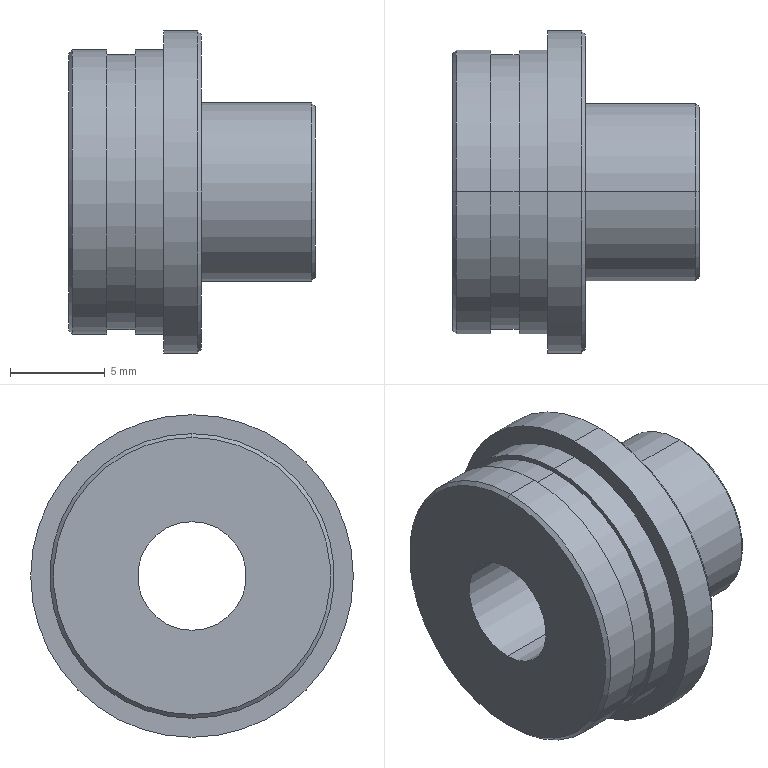Part | SolidWorks | features BaseBody 1 | 1 solid | 24 faces | box 13 x 17 x 17 mm | volume 1399 mm3 | cylinder 12 | cone 6 | plane 6 | commonest cylinder face diameters 15 x4 5.729 x2 9.4 x2 14.5 x2 17 x2
STEP:
#1=CARTESIAN_POINT('',(0.,0.,4.7));
#2=VERTEX_POINT('',#1);
#3=CARTESIAN_POINT('',(0.,0.,-4.7));
#4=VERTEX_POINT('',#3);
#5=CARTESIAN_POINT('',(0.,0.,0.));
#6=DIRECTION('',(-1.,0.,0.));
#7=DIRECTION('',(0.,0.,-1.));
#8=AXIS2_PLACEMENT_3D('',#5,#6,#7);
#9=CIRCLE('',#8,4.7);
#10=EDGE_CURVE('',#2,#4,#9,.T.);
#11=ORIENTED_EDGE('',*,*,#10,.F.);
#12=CARTESIAN_POINT('',(5.8,0.,4.7));
#13=VERTEX_POINT('',#12);
#14=CARTESIAN_POINT('',(0.,0.,4.7));
#15=DIRECTION('',(1.,0.,0.));
#16=VECTOR('',#15,1000.);
#17=LINE('',#14,#16);
#18=EDGE_CURVE('',#2,#13,#17,.T.);
#19=ORIENTED_EDGE('',*,*,#18,.T.);
#20=CARTESIAN_POINT('',(5.8,0.,-4.7));
#21=VERTEX_POINT('',#20);
#22=CARTESIAN_POINT('',(5.8,0.,0.));
#23=DIRECTION('',(-1.,0.,0.));
#24=DIRECTION('',(0.,0.,-1.));
#25=AXIS2_PLACEMENT_3D('',#22,#23,#24);
#26=CIRCLE('',#25,4.7);
#27=EDGE_CURVE('',#13,#21,#26,.T.);
#28=ORIENTED_EDGE('',*,*,#27,.T.);
#29=CARTESIAN_POINT('',(0.,0.,-4.7));
#30=DIRECTION('',(1.,0.,0.));
#31=VECTOR('',#30,1000.);
#32=LINE('',#29,#31);
#33=EDGE_CURVE('',#4,#21,#32,.T.);
#34=ORIENTED_EDGE('',*,*,#33,.F.);
#35=EDGE_LOOP('',(#11,#19,#28,#34));
#36=FACE_OUTER_BOUND('',#35,.T.);
#37=CARTESIAN_POINT('',(0.,0.,0.));
#38=DIRECTION('',(1.,0.,0.));
#39=DIRECTION('',(0.,0.,-1.));
#40=AXIS2_PLACEMENT_3D('',#37,#38,#39);
#41=CYLINDRICAL_SURFACE('',#40,4.7);
#42=ADVANCED_FACE('',(#36),#41,.T.);
#43=CARTESIAN_POINT('',(0.,0.,-8.3));
#44=VERTEX_POINT('',#43);
#45=CARTESIAN_POINT('',(0.,0.,8.3));
#46=VERTEX_POINT('',#45);
#47=CARTESIAN_POINT('',(0.,0.,0.));
#48=DIRECTION('',(1.,0.,0.));
#49=DIRECTION('',(0.,0.,1.));
#50=AXIS2_PLACEMENT_3D('',#47,#48,#49);
#51=CIRCLE('',#50,8.3);
#52=EDGE_CURVE('',#44,#46,#51,.T.);
#53=ORIENTED_EDGE('',*,*,#52,.F.);
#54=CARTESIAN_POINT('',(-0.2,0.,-8.5));
#55=VERTEX_POINT('',#54);
#56=CARTESIAN_POINT('',(-0.2,0.,-8.5));
#57=DIRECTION('',(-0.7071,0.,-0.7071));
#58=VECTOR('',#57,1000.);
#59=LINE('',#56,#58);
#60=EDGE_CURVE('',#44,#55,#59,.T.);
#61=ORIENTED_EDGE('',*,*,#60,.T.);
#62=CARTESIAN_POINT('',(-0.2,0.,8.5));
#63=VERTEX_POINT('',#62);
#64=CARTESIAN_POINT('',(-0.2,0.,0.));
#65=DIRECTION('',(1.,0.,0.));
#66=DIRECTION('',(0.,0.,1.));
#67=AXIS2_PLACEMENT_3D('',#64,#65,#66);
#68=CIRCLE('',#67,8.5);
#69=EDGE_CURVE('',#55,#63,#68,.T.);
#70=ORIENTED_EDGE('',*,*,#69,.T.);
#71=CARTESIAN_POINT('',(-0.2,0.,8.5));
#72=DIRECTION('',(-0.7071,0.,0.7071));
#73=VECTOR('',#72,1000.);
#74=LINE('',#71,#73);
#75=EDGE_CURVE('',#46,#63,#74,.T.);
#76=ORIENTED_EDGE('',*,*,#75,.F.);
#77=EDGE_LOOP('',(#53,#61,#70,#76));
#78=FACE_OUTER_BOUND('',#77,.T.);
#79=CARTESIAN_POINT('',(-0.2,0.,0.));
#80=DIRECTION('',(-1.,0.,0.));
#81=DIRECTION('',(0.,0.,1.));
#82=AXIS2_PLACEMENT_3D('',#79,#80,#81);
#83=CONICAL_SURFACE('',#82,8.5,0.7854);
#84=ADVANCED_FACE('',(#78),#83,.T.);
#85=CARTESIAN_POINT('',(6.,0.,4.5));
#86=VERTEX_POINT('',#85);
#87=CARTESIAN_POINT('',(6.,0.,-4.5));
#88=VERTEX_POINT('',#87);
#89=CARTESIAN_POINT('',(6.,0.,0.));
#90=DIRECTION('',(-1.,0.,0.));
#91=DIRECTION('',(0.,0.,1.));
#92=AXIS2_PLACEMENT_3D('',#89,#90,#91);
#93=CIRCLE('',#92,4.5);
#94=EDGE_CURVE('',#86,#88,#93,.T.);
#95=ORIENTED_EDGE('',*,*,#94,.T.);
#96=CARTESIAN_POINT('',(5.8,0.,-4.7));
#97=DIRECTION('',(-0.7071,0.,-0.7071));
#98=VECTOR('',#97,1000.);
#99=LINE('',#96,#98);
#100=EDGE_CURVE('',#88,#21,#99,.T.);
#101=ORIENTED_EDGE('',*,*,#100,.T.);
#102=ORIENTED_EDGE('',*,*,#27,.F.);
#103=CARTESIAN_POINT('',(5.8,0.,4.7));
#104=DIRECTION('',(-0.7071,0.,0.7071));
#105=VECTOR('',#104,1000.);
#106=LINE('',#103,#105);
#107=EDGE_CURVE('',#86,#13,#106,.T.);
#108=ORIENTED_EDGE('',*,*,#107,.F.);
#109=EDGE_LOOP('',(#95,#101,#102,#108));
#110=FACE_OUTER_BOUND('',#109,.T.);
#111=CARTESIAN_POINT('',(5.8,0.,0.));
#112=DIRECTION('',(-1.,0.,0.));
#113=DIRECTION('',(0.,0.,1.));
#114=AXIS2_PLACEMENT_3D('',#111,#112,#113);
#115=CONICAL_SURFACE('',#114,4.7,0.7854);
#116=ADVANCED_FACE('',(#110),#115,.T.);
#117=CARTESIAN_POINT('',(-2.,0.,-8.5));
#118=VERTEX_POINT('',#117);
#119=CARTESIAN_POINT('',(-2.,0.,8.5));
#120=VERTEX_POINT('',#119);
#121=CARTESIAN_POINT('',(-2.,0.,0.));
#122=DIRECTION('',(1.,0.,0.));
#123=DIRECTION('',(0.,0.,-1.));
#124=AXIS2_PLACEMENT_3D('',#121,#122,#123);
#125=CIRCLE('',#124,8.5);
#126=EDGE_CURVE('',#118,#120,#125,.T.);
#127=ORIENTED_EDGE('',*,*,#126,.T.);
#128=CARTESIAN_POINT('',(0.,0.,8.5));
#129=DIRECTION('',(1.,0.,0.));
#130=VECTOR('',#129,1000.);
#131=LINE('',#128,#130);
#132=EDGE_CURVE('',#120,#63,#131,.T.);
#133=ORIENTED_EDGE('',*,*,#132,.T.);
#134=ORIENTED_EDGE('',*,*,#69,.F.);
#135=CARTESIAN_POINT('',(0.,0.,-8.5));
#136=DIRECTION('',(1.,0.,0.));
#137=VECTOR('',#136,1000.);
#138=LINE('',#135,#137);
#139=EDGE_CURVE('',#118,#55,#138,.T.);
#140=ORIENTED_EDGE('',*,*,#139,.F.);
#141=EDGE_LOOP('',(#127,#133,#134,#140));
#142=FACE_OUTER_BOUND('',#141,.T.);
#143=CARTESIAN_POINT('',(0.,0.,0.));
#144=DIRECTION('',(1.,0.,0.));
#145=DIRECTION('',(0.,0.,-1.));
#146=AXIS2_PLACEMENT_3D('',#143,#144,#145);
#147=CYLINDRICAL_SURFACE('',#146,8.5);
#148=ADVANCED_FACE('',(#142),#147,.T.);
#149=CARTESIAN_POINT('',(-7.,0.,2.864));
#150=VERTEX_POINT('',#149);
#151=CARTESIAN_POINT('',(-7.,0.,-2.864));
#152=VERTEX_POINT('',#151);
#153=CARTESIAN_POINT('',(-7.,0.,0.));
#154=DIRECTION('',(1.,0.,0.));
#155=DIRECTION('',(0.,0.,-1.));
#156=AXIS2_PLACEMENT_3D('',#153,#154,#155);
#157=CIRCLE('',#156,2.864);
#158=EDGE_CURVE('',#150,#152,#157,.T.);
#159=ORIENTED_EDGE('',*,*,#158,.F.);
#160=CARTESIAN_POINT('',(6.,0.,2.864));
#161=VERTEX_POINT('',#160);
#162=CARTESIAN_POINT('',(0.,0.,2.864));
#163=DIRECTION('',(1.,0.,0.));
#164=VECTOR('',#163,1000.);
#165=LINE('',#162,#164);
#166=EDGE_CURVE('',#150,#161,#165,.T.);
#167=ORIENTED_EDGE('',*,*,#166,.T.);
#168=CARTESIAN_POINT('',(6.,0.,-2.864));
#169=VERTEX_POINT('',#168);
#170=CARTESIAN_POINT('',(6.,0.,0.));
#171=DIRECTION('',(-1.,0.,0.));
#172=DIRECTION('',(0.,0.,-1.));
#173=AXIS2_PLACEMENT_3D('',#170,#171,#172);
#174=CIRCLE('',#173,2.864);
#175=EDGE_CURVE('',#169,#161,#174,.T.);
#176=ORIENTED_EDGE('',*,*,#175,.F.);
#177=CARTESIAN_POINT('',(0.,0.,-2.864));
#178=DIRECTION('',(1.,0.,0.));
#179=VECTOR('',#178,1000.);
#180=LINE('',#177,#179);
#181=EDGE_CURVE('',#152,#169,#180,.T.);
#182=ORIENTED_EDGE('',*,*,#181,.F.);
#183=EDGE_LOOP('',(#159,#167,#176,#182));
#184=FACE_OUTER_BOUND('',#183,.T.);
#185=CARTESIAN_POINT('',(0.,0.,0.));
#186=DIRECTION('',(1.,0.,0.));
#187=DIRECTION('',(0.,0.,-1.));
#188=AXIS2_PLACEMENT_3D('',#185,#186,#187);
#189=CYLINDRICAL_SURFACE('',#188,2.864);
#190=ADVANCED_FACE('',(#184),#189,.F.);
#191=CARTESIAN_POINT('',(-3.5,0.,-7.5));
#192=VERTEX_POINT('',#191);
#193=CARTESIAN_POINT('',(-3.5,0.,7.5));
#194=VERTEX_POINT('',#193);
#195=CARTESIAN_POINT('',(-3.5,0.,0.));
#196=DIRECTION('',(1.,0.,0.));
#197=DIRECTION('',(0.,0.,-1.));
#198=AXIS2_PLACEMENT_3D('',#195,#196,#197);
#199=CIRCLE('',#198,7.5);
#200=EDGE_CURVE('',#192,#194,#199,.T.);
#201=ORIENTED_EDGE('',*,*,#200,.T.);
#202=CARTESIAN_POINT('',(-2.,0.,7.5));
#203=VERTEX_POINT('',#202);
#204=CARTESIAN_POINT('',(0.,0.,7.5));
#205=DIRECTION('',(1.,0.,0.));
#206=VECTOR('',#205,1000.);
#207=LINE('',#204,#206);
#208=EDGE_CURVE('',#194,#203,#207,.T.);
#209=ORIENTED_EDGE('',*,*,#208,.T.);
#210=CARTESIAN_POINT('',(-2.,0.,-7.5));
#211=VERTEX_POINT('',#210);
#212=CARTESIAN_POINT('',(-2.,0.,0.));
#213=DIRECTION('',(1.,0.,0.));
#214=DIRECTION('',(0.,0.,-1.));
#215=AXIS2_PLACEMENT_3D('',#212,#213,#214);
#216=CIRCLE('',#215,7.5);
#217=EDGE_CURVE('',#211,#203,#216,.T.);
#218=ORIENTED_EDGE('',*,*,#217,.F.);
#219=CARTESIAN_POINT('',(0.,0.,-7.5));
#220=DIRECTION('',(1.,0.,0.));
#221=VECTOR('',#220,1000.);
#222=LINE('',#219,#221);
#223=EDGE_CURVE('',#192,#211,#222,.T.);
#224=ORIENTED_EDGE('',*,*,#223,.F.);
#225=EDGE_LOOP('',(#201,#209,#218,#224));
#226=FACE_OUTER_BOUND('',#225,.T.);
#227=CARTESIAN_POINT('',(0.,0.,0.));
#228=DIRECTION('',(1.,0.,0.));
#229=DIRECTION('',(0.,0.,-1.));
#230=AXIS2_PLACEMENT_3D('',#227,#228,#229);
#231=CYLINDRICAL_SURFACE('',#230,7.5);
#232=ADVANCED_FACE('',(#226),#231,.T.);
#233=CARTESIAN_POINT('',(-7.,0.,7.3));
#234=VERTEX_POINT('',#233);
#235=CARTESIAN_POINT('',(-7.,0.,-7.3));
#236=VERTEX_POINT('',#235);
#237=CARTESIAN_POINT('',(-7.,0.,0.));
#238=DIRECTION('',(-1.,0.,0.));
#239=DIRECTION('',(0.,0.,-1.));
#240=AXIS2_PLACEMENT_3D('',#237,#238,#239);
#241=CIRCLE('',#240,7.3);
#242=EDGE_CURVE('',#234,#236,#241,.T.);
#243=ORIENTED_EDGE('',*,*,#242,.F.);
#244=CARTESIAN_POINT('',(-6.8,0.,7.5));
#245=VERTEX_POINT('',#244);
#246=CARTESIAN_POINT('',(-6.8,0.,7.5));
#247=DIRECTION('',(0.7071,0.,0.7071));
#248=VECTOR('',#247,1000.);
#249=LINE('',#246,#248);
#250=EDGE_CURVE('',#234,#245,#249,.T.);
#251=ORIENTED_EDGE('',*,*,#250,.T.);
#252=CARTESIAN_POINT('',(-6.8,0.,-7.5));
#253=VERTEX_POINT('',#252);
#254=CARTESIAN_POINT('',(-6.8,0.,0.));
#255=DIRECTION('',(-1.,0.,0.));
#256=DIRECTION('',(0.,0.,-1.));
#257=AXIS2_PLACEMENT_3D('',#254,#255,#256);
#258=CIRCLE('',#257,7.5);
#259=EDGE_CURVE('',#245,#253,#258,.T.);
#260=ORIENTED_EDGE('',*,*,#259,.T.);
#261=CARTESIAN_POINT('',(-6.8,0.,-7.5));
#262=DIRECTION('',(0.7071,0.,-0.7071));
#263=VECTOR('',#262,1000.);
#264=LINE('',#261,#263);
#265=EDGE_CURVE('',#236,#253,#264,.T.);
#266=ORIENTED_EDGE('',*,*,#265,.F.);
#267=EDGE_LOOP('',(#243,#251,#260,#266));
#268=FACE_OUTER_BOUND('',#267,.T.);
#269=CARTESIAN_POINT('',(-6.8,0.,0.));
#270=DIRECTION('',(1.,0.,0.));
#271=DIRECTION('',(0.,0.,-1.));
#272=AXIS2_PLACEMENT_3D('',#269,#270,#271);
#273=CONICAL_SURFACE('',#272,7.5,0.7854);
#274=ADVANCED_FACE('',(#268),#273,.T.);
#275=CARTESIAN_POINT('',(-5.,0.,-7.25));
#276=VERTEX_POINT('',#275);
#277=CARTESIAN_POINT('',(-5.,0.,7.25));
#278=VERTEX_POINT('',#277);
#279=CARTESIAN_POINT('',(-5.,0.,0.));
#280=DIRECTION('',(1.,0.,0.));
#281=DIRECTION('',(0.,0.,-1.));
#282=AXIS2_PLACEMENT_3D('',#279,#280,#281);
#283=CIRCLE('',#282,7.25);
#284=EDGE_CURVE('',#276,#278,#283,.T.);
#285=ORIENTED_EDGE('',*,*,#284,.T.);
#286=CARTESIAN_POINT('',(-3.5,0.,7.25));
#287=VERTEX_POINT('',#286);
#288=CARTESIAN_POINT('',(0.,0.,7.25));
#289=DIRECTION('',(1.,0.,0.));
#290=VECTOR('',#289,1000.);
#291=LINE('',#288,#290);
#292=EDGE_CURVE('',#278,#287,#291,.T.);
#293=ORIENTED_EDGE('',*,*,#292,.T.);
#294=CARTESIAN_POINT('',(-3.5,0.,-7.25));
#295=VERTEX_POINT('',#294);
#296=CARTESIAN_POINT('',(-3.5,0.,0.));
#297=DIRECTION('',(1.,0.,0.));
#298=DIRECTION('',(0.,0.,-1.));
#299=AXIS2_PLACEMENT_3D('',#296,#297,#298);
#300=CIRCLE('',#299,7.25);
#301=EDGE_CURVE('',#295,#287,#300,.T.);
#302=ORIENTED_EDGE('',*,*,#301,.F.);
#303=CARTESIAN_POINT('',(0.,0.,-7.25));
#304=DIRECTION('',(1.,0.,0.));
#305=VECTOR('',#304,1000.);
#306=LINE('',#303,#305);
#307=EDGE_CURVE('',#276,#295,#306,.T.);
#308=ORIENTED_EDGE('',*,*,#307,.F.);
#309=EDGE_LOOP('',(#285,#293,#302,#308));
#310=FACE_OUTER_BOUND('',#309,.T.);
#311=CARTESIAN_POINT('',(0.,0.,0.));
#312=DIRECTION('',(1.,0.,0.));
#313=DIRECTION('',(0.,0.,-1.));
#314=AXIS2_PLACEMENT_3D('',#311,#312,#313);
#315=CYLINDRICAL_SURFACE('',#314,7.25);
#316=ADVANCED_FACE('',(#310),#315,.T.);
#317=ORIENTED_EDGE('',*,*,#259,.F.);
#318=CARTESIAN_POINT('',(-5.,0.,7.5));
#319=VERTEX_POINT('',#318);
#320=CARTESIAN_POINT('',(0.,0.,7.5));
#321=DIRECTION('',(1.,0.,0.));
#322=VECTOR('',#321,1000.);
#323=LINE('',#320,#322);
#324=EDGE_CURVE('',#245,#319,#323,.T.);
#325=ORIENTED_EDGE('',*,*,#324,.T.);
#326=CARTESIAN_POINT('',(-5.,0.,-7.5));
#327=VERTEX_POINT('',#326);
#328=CARTESIAN_POINT('',(-5.,0.,0.));
#329=DIRECTION('',(-1.,0.,0.));
#330=DIRECTION('',(0.,0.,-1.));
#331=AXIS2_PLACEMENT_3D('',#328,#329,#330);
#332=CIRCLE('',#331,7.5);
#333=EDGE_CURVE('',#319,#327,#332,.T.);
#334=ORIENTED_EDGE('',*,*,#333,.T.);
#335=CARTESIAN_POINT('',(0.,0.,-7.5));
#336=DIRECTION('',(1.,0.,0.));
#337=VECTOR('',#336,1000.);
#338=LINE('',#335,#337);
#339=EDGE_CURVE('',#253,#327,#338,.T.);
#340=ORIENTED_EDGE('',*,*,#339,.F.);
#341=EDGE_LOOP('',(#317,#325,#334,#340));
#342=FACE_OUTER_BOUND('',#341,.T.);
#343=CARTESIAN_POINT('',(0.,0.,0.));
#344=DIRECTION('',(1.,0.,0.));
#345=DIRECTION('',(0.,0.,-1.));
#346=AXIS2_PLACEMENT_3D('',#343,#344,#345);
#347=CYLINDRICAL_SURFACE('',#346,7.5);
#348=ADVANCED_FACE('',(#342),#347,.T.);
#349=CARTESIAN_POINT('',(0.,0.,0.));
#350=DIRECTION('',(-1.,0.,0.));
#351=DIRECTION('',(0.,0.,-1.));
#352=AXIS2_PLACEMENT_3D('',#349,#350,#351);
#353=CIRCLE('',#352,4.7);
#354=EDGE_CURVE('',#4,#2,#353,.T.);
#355=ORIENTED_EDGE('',*,*,#354,.T.);
#356=ORIENTED_EDGE('',*,*,#10,.T.);
#357=EDGE_LOOP('',(#355,#356));
#358=FACE_BOUND('',#357,.T.);
#359=CARTESIAN_POINT('',(0.,0.,0.));
#360=DIRECTION('',(1.,0.,0.));
#361=DIRECTION('',(0.,0.,1.));
#362=AXIS2_PLACEMENT_3D('',#359,#360,#361);
#363=CIRCLE('',#362,8.3);
#364=EDGE_CURVE('',#46,#44,#363,.T.);
#365=ORIENTED_EDGE('',*,*,#364,.T.);
#366=ORIENTED_EDGE('',*,*,#52,.T.);
#367=EDGE_LOOP('',(#365,#366));
#368=FACE_OUTER_BOUND('',#367,.T.);
#369=CARTESIAN_POINT('',(0.,4.7,0.));
#370=DIRECTION('',(1.,0.,0.));
#371=DIRECTION('',(0.,0.,-1.));
#372=AXIS2_PLACEMENT_3D('',#369,#370,#371);
#373=PLANE('',#372);
#374=ADVANCED_FACE('',(#358,#368),#373,.T.);
#375=ORIENTED_EDGE('',*,*,#18,.F.);
#376=ORIENTED_EDGE('',*,*,#354,.F.);
#377=ORIENTED_EDGE('',*,*,#33,.T.);
#378=CARTESIAN_POINT('',(5.8,0.,0.));
#379=DIRECTION('',(-1.,0.,0.));
#380=DIRECTION('',(0.,0.,-1.));
#381=AXIS2_PLACEMENT_3D('',#378,#379,#380);
#382=CIRCLE('',#381,4.7);
#383=EDGE_CURVE('',#21,#13,#382,.T.);
#384=ORIENTED_EDGE('',*,*,#383,.T.);
#385=EDGE_LOOP('',(#375,#376,#377,#384));
#386=FACE_OUTER_BOUND('',#385,.T.);
#387=CARTESIAN_POINT('',(0.,0.,0.));
#388=DIRECTION('',(1.,0.,0.));
#389=DIRECTION('',(0.,0.,-1.));
#390=AXIS2_PLACEMENT_3D('',#387,#388,#389);
#391=CYLINDRICAL_SURFACE('',#390,4.7);
#392=ADVANCED_FACE('',(#386),#391,.T.);
#393=ORIENTED_EDGE('',*,*,#60,.F.);
#394=ORIENTED_EDGE('',*,*,#364,.F.);
#395=ORIENTED_EDGE('',*,*,#75,.T.);
#396=CARTESIAN_POINT('',(-0.2,0.,0.));
#397=DIRECTION('',(1.,0.,0.));
#398=DIRECTION('',(0.,0.,1.));
#399=AXIS2_PLACEMENT_3D('',#396,#397,#398);
#400=CIRCLE('',#399,8.5);
#401=EDGE_CURVE('',#63,#55,#400,.T.);
#402=ORIENTED_EDGE('',*,*,#401,.T.);
#403=EDGE_LOOP('',(#393,#394,#395,#402));
#404=FACE_OUTER_BOUND('',#403,.T.);
#405=CARTESIAN_POINT('',(-0.2,0.,0.));
#406=DIRECTION('',(-1.,0.,0.));
#407=DIRECTION('',(0.,0.,1.));
#408=AXIS2_PLACEMENT_3D('',#405,#406,#407);
#409=CONICAL_SURFACE('',#408,8.5,0.7854);
#410=ADVANCED_FACE('',(#404),#409,.T.);
#411=ORIENTED_EDGE('',*,*,#100,.F.);
#412=CARTESIAN_POINT('',(6.,0.,0.));
#413=DIRECTION('',(-1.,0.,0.));
#414=DIRECTION('',(0.,0.,1.));
#415=AXIS2_PLACEMENT_3D('',#412,#413,#414);
#416=CIRCLE('',#415,4.5);
#417=EDGE_CURVE('',#88,#86,#416,.T.);
#418=ORIENTED_EDGE('',*,*,#417,.T.);
#419=ORIENTED_EDGE('',*,*,#107,.T.);
#420=ORIENTED_EDGE('',*,*,#383,.F.);
#421=EDGE_LOOP('',(#411,#418,#419,#420));
#422=FACE_OUTER_BOUND('',#421,.T.);
#423=CARTESIAN_POINT('',(5.8,0.,0.));
#424=DIRECTION('',(-1.,0.,0.));
#425=DIRECTION('',(0.,0.,1.));
#426=AXIS2_PLACEMENT_3D('',#423,#424,#425);
#427=CONICAL_SURFACE('',#426,4.7,0.7854);
#428=ADVANCED_FACE('',(#422),#427,.T.);
#429=ORIENTED_EDGE('',*,*,#132,.F.);
#430=CARTESIAN_POINT('',(-2.,0.,0.));
#431=DIRECTION('',(1.,0.,0.));
#432=DIRECTION('',(0.,0.,-1.));
#433=AXIS2_PLACEMENT_3D('',#430,#431,#432);
#434=CIRCLE('',#433,8.5);
#435=EDGE_CURVE('',#120,#118,#434,.T.);
#436=ORIENTED_EDGE('',*,*,#435,.T.);
#437=ORIENTED_EDGE('',*,*,#139,.T.);
#438=ORIENTED_EDGE('',*,*,#401,.F.);
#439=EDGE_LOOP('',(#429,#436,#437,#438));
#440=FACE_OUTER_BOUND('',#439,.T.);
#441=CARTESIAN_POINT('',(0.,0.,0.));
#442=DIRECTION('',(1.,0.,0.));
#443=DIRECTION('',(0.,0.,-1.));
#444=AXIS2_PLACEMENT_3D('',#441,#442,#443);
#445=CYLINDRICAL_SURFACE('',#444,8.5);
#446=ADVANCED_FACE('',(#440),#445,.T.);
#447=ORIENTED_EDGE('',*,*,#175,.T.);
#448=CARTESIAN_POINT('',(6.,0.,0.));
#449=DIRECTION('',(-1.,0.,0.));
#450=DIRECTION('',(0.,0.,-1.));
#451=AXIS2_PLACEMENT_3D('',#448,#449,#450);
#452=CIRCLE('',#451,2.864);
#453=EDGE_CURVE('',#161,#169,#452,.T.);
#454=ORIENTED_EDGE('',*,*,#453,.T.);
#455=EDGE_LOOP('',(#447,#454));
#456=FACE_BOUND('',#455,.T.);
#457=ORIENTED_EDGE('',*,*,#94,.F.);
#458=ORIENTED_EDGE('',*,*,#417,.F.);
#459=EDGE_LOOP('',(#457,#458));
#460=FACE_OUTER_BOUND('',#459,.T.);
#461=CARTESIAN_POINT('',(6.,4.7,0.));
#462=DIRECTION('',(1.,0.,0.));
#463=DIRECTION('',(0.,0.,-1.));
#464=AXIS2_PLACEMENT_3D('',#461,#462,#463);
#465=PLANE('',#464);
#466=ADVANCED_FACE('',(#456,#460),#465,.T.);
#467=ORIENTED_EDGE('',*,*,#126,.F.);
#468=ORIENTED_EDGE('',*,*,#435,.F.);
#469=EDGE_LOOP('',(#467,#468));
#470=FACE_OUTER_BOUND('',#469,.T.);
#471=ORIENTED_EDGE('',*,*,#217,.T.);
#472=CARTESIAN_POINT('',(-2.,0.,0.));
#473=DIRECTION('',(1.,0.,0.));
#474=DIRECTION('',(0.,0.,-1.));
#475=AXIS2_PLACEMENT_3D('',#472,#473,#474);
#476=CIRCLE('',#475,7.5);
#477=EDGE_CURVE('',#203,#211,#476,.T.);
#478=ORIENTED_EDGE('',*,*,#477,.T.);
#479=EDGE_LOOP('',(#471,#478));
#480=FACE_BOUND('',#479,.T.);
#481=CARTESIAN_POINT('',(-2.,8.5,0.));
#482=DIRECTION('',(-1.,0.,0.));
#483=DIRECTION('',(0.,0.,1.));
#484=AXIS2_PLACEMENT_3D('',#481,#482,#483);
#485=PLANE('',#484);
#486=ADVANCED_FACE('',(#470,#480),#485,.T.);
#487=ORIENTED_EDGE('',*,*,#166,.F.);
#488=CARTESIAN_POINT('',(-7.,0.,0.));
#489=DIRECTION('',(1.,0.,0.));
#490=DIRECTION('',(0.,0.,-1.));
#491=AXIS2_PLACEMENT_3D('',#488,#489,#490);
#492=CIRCLE('',#491,2.864);
#493=EDGE_CURVE('',#152,#150,#492,.T.);
#494=ORIENTED_EDGE('',*,*,#493,.F.);
#495=ORIENTED_EDGE('',*,*,#181,.T.);
#496=ORIENTED_EDGE('',*,*,#453,.F.);
#497=EDGE_LOOP('',(#487,#494,#495,#496));
#498=FACE_OUTER_BOUND('',#497,.T.);
#499=CARTESIAN_POINT('',(0.,0.,0.));
#500=DIRECTION('',(1.,0.,0.));
#501=DIRECTION('',(0.,0.,-1.));
#502=AXIS2_PLACEMENT_3D('',#499,#500,#501);
#503=CYLINDRICAL_SURFACE('',#502,2.864);
#504=ADVANCED_FACE('',(#498),#503,.F.);
#505=ORIENTED_EDGE('',*,*,#208,.F.);
#506=CARTESIAN_POINT('',(-3.5,0.,0.));
#507=DIRECTION('',(1.,0.,0.));
#508=DIRECTION('',(0.,0.,-1.));
#509=AXIS2_PLACEMENT_3D('',#506,#507,#508);
#510=CIRCLE('',#509,7.5);
#511=EDGE_CURVE('',#194,#192,#510,.T.);
#512=ORIENTED_EDGE('',*,*,#511,.T.);
#513=ORIENTED_EDGE('',*,*,#223,.T.);
#514=ORIENTED_EDGE('',*,*,#477,.F.);
#515=EDGE_LOOP('',(#505,#512,#513,#514));
#516=FACE_OUTER_BOUND('',#515,.T.);
#517=CARTESIAN_POINT('',(0.,0.,0.));
#518=DIRECTION('',(1.,0.,0.));
#519=DIRECTION('',(0.,0.,-1.));
#520=AXIS2_PLACEMENT_3D('',#517,#518,#519);
#521=CYLINDRICAL_SURFACE('',#520,7.5);
#522=ADVANCED_FACE('',(#516),#521,.T.);
#523=ORIENTED_EDGE('',*,*,#493,.T.);
#524=ORIENTED_EDGE('',*,*,#158,.T.);
#525=EDGE_LOOP('',(#523,#524));
#526=FACE_BOUND('',#525,.T.);
#527=CARTESIAN_POINT('',(-7.,0.,0.));
#528=DIRECTION('',(-1.,0.,0.));
#529=DIRECTION('',(0.,0.,-1.));
#530=AXIS2_PLACEMENT_3D('',#527,#528,#529);
#531=CIRCLE('',#530,7.3);
#532=EDGE_CURVE('',#236,#234,#531,.T.);
#533=ORIENTED_EDGE('',*,*,#532,.T.);
#534=ORIENTED_EDGE('',*,*,#242,.T.);
#535=EDGE_LOOP('',(#533,#534));
#536=FACE_OUTER_BOUND('',#535,.T.);
#537=CARTESIAN_POINT('',(-7.,7.5,0.));
#538=DIRECTION('',(-1.,0.,0.));
#539=DIRECTION('',(0.,0.,1.));
#540=AXIS2_PLACEMENT_3D('',#537,#538,#539);
#541=PLANE('',#540);
#542=ADVANCED_FACE('',(#526,#536),#541,.T.);
#543=ORIENTED_EDGE('',*,*,#200,.F.);
#544=ORIENTED_EDGE('',*,*,#511,.F.);
#545=EDGE_LOOP('',(#543,#544));
#546=FACE_OUTER_BOUND('',#545,.T.);
#547=ORIENTED_EDGE('',*,*,#301,.T.);
#548=CARTESIAN_POINT('',(-3.5,0.,0.));
#549=DIRECTION('',(1.,0.,0.));
#550=DIRECTION('',(0.,0.,-1.));
#551=AXIS2_PLACEMENT_3D('',#548,#549,#550);
#552=CIRCLE('',#551,7.25);
#553=EDGE_CURVE('',#287,#295,#552,.T.);
#554=ORIENTED_EDGE('',*,*,#553,.T.);
#555=EDGE_LOOP('',(#547,#554));
#556=FACE_BOUND('',#555,.T.);
#557=CARTESIAN_POINT('',(-3.5,7.5,0.));
#558=DIRECTION('',(-1.,0.,0.));
#559=DIRECTION('',(0.,0.,1.));
#560=AXIS2_PLACEMENT_3D('',#557,#558,#559);
#561=PLANE('',#560);
#562=ADVANCED_FACE('',(#546,#556),#561,.T.);
#563=ORIENTED_EDGE('',*,*,#250,.F.);
#564=ORIENTED_EDGE('',*,*,#532,.F.);
#565=ORIENTED_EDGE('',*,*,#265,.T.);
#566=CARTESIAN_POINT('',(-6.8,0.,0.));
#567=DIRECTION('',(-1.,0.,0.));
#568=DIRECTION('',(0.,0.,-1.));
#569=AXIS2_PLACEMENT_3D('',#566,#567,#568);
#570=CIRCLE('',#569,7.5);
#571=EDGE_CURVE('',#253,#245,#570,.T.);
#572=ORIENTED_EDGE('',*,*,#571,.T.);
#573=EDGE_LOOP('',(#563,#564,#565,#572));
#574=FACE_OUTER_BOUND('',#573,.T.);
#575=CARTESIAN_POINT('',(-6.8,0.,0.));
#576=DIRECTION('',(1.,0.,0.));
#577=DIRECTION('',(0.,0.,-1.));
#578=AXIS2_PLACEMENT_3D('',#575,#576,#577);
#579=CONICAL_SURFACE('',#578,7.5,0.7854);
#580=ADVANCED_FACE('',(#574),#579,.T.);
#581=ORIENTED_EDGE('',*,*,#292,.F.);
#582=CARTESIAN_POINT('',(-5.,0.,0.));
#583=DIRECTION('',(1.,0.,0.));
#584=DIRECTION('',(0.,0.,-1.));
#585=AXIS2_PLACEMENT_3D('',#582,#583,#584);
#586=CIRCLE('',#585,7.25);
#587=EDGE_CURVE('',#278,#276,#586,.T.);
#588=ORIENTED_EDGE('',*,*,#587,.T.);
#589=ORIENTED_EDGE('',*,*,#307,.T.);
#590=ORIENTED_EDGE('',*,*,#553,.F.);
#591=EDGE_LOOP('',(#581,#588,#589,#590));
#592=FACE_OUTER_BOUND('',#591,.T.);
#593=CARTESIAN_POINT('',(0.,0.,0.));
#594=DIRECTION('',(1.,0.,0.));
#595=DIRECTION('',(0.,0.,-1.));
#596=AXIS2_PLACEMENT_3D('',#593,#594,#595);
#597=CYLINDRICAL_SURFACE('',#596,7.25);
#598=ADVANCED_FACE('',(#592),#597,.T.);
#599=ORIENTED_EDGE('',*,*,#324,.F.);
#600=ORIENTED_EDGE('',*,*,#571,.F.);
#601=ORIENTED_EDGE('',*,*,#339,.T.);
#602=CARTESIAN_POINT('',(-5.,0.,0.));
#603=DIRECTION('',(-1.,0.,0.));
#604=DIRECTION('',(0.,0.,-1.));
#605=AXIS2_PLACEMENT_3D('',#602,#603,#604);
#606=CIRCLE('',#605,7.5);
#607=EDGE_CURVE('',#327,#319,#606,.T.);
#608=ORIENTED_EDGE('',*,*,#607,.T.);
#609=EDGE_LOOP('',(#599,#600,#601,#608));
#610=FACE_OUTER_BOUND('',#609,.T.);
#611=CARTESIAN_POINT('',(0.,0.,0.));
#612=DIRECTION('',(1.,0.,0.));
#613=DIRECTION('',(0.,0.,-1.));
#614=AXIS2_PLACEMENT_3D('',#611,#612,#613);
#615=CYLINDRICAL_SURFACE('',#614,7.5);
#616=ADVANCED_FACE('',(#610),#615,.T.);
#617=ORIENTED_EDGE('',*,*,#284,.F.);
#618=ORIENTED_EDGE('',*,*,#587,.F.);
#619=EDGE_LOOP('',(#617,#618));
#620=FACE_BOUND('',#619,.T.);
#621=ORIENTED_EDGE('',*,*,#607,.F.);
#622=ORIENTED_EDGE('',*,*,#333,.F.);
#623=EDGE_LOOP('',(#621,#622));
#624=FACE_OUTER_BOUND('',#623,.T.);
#625=CARTESIAN_POINT('',(-5.,7.25,0.));
#626=DIRECTION('',(1.,0.,0.));
#627=DIRECTION('',(0.,0.,-1.));
#628=AXIS2_PLACEMENT_3D('',#625,#626,#627);
#629=PLANE('',#628);
#630=ADVANCED_FACE('',(#620,#624),#629,.T.);
#631=CLOSED_SHELL('',(#42,#84,#116,#148,#190,#232,#274,#316,#348,#374,#392,#410,#428,#446,#466,#486,#504,#522,#542,#562,#580,#598,#616,#630));
#632=MANIFOLD_SOLID_BREP('',#631);
#633=CARTESIAN_POINT('',(0.,0.,0.));
#634=DIRECTION('',(0.,0.,1.));
#635=DIRECTION('',(1.,0.,0.));
#636=AXIS2_PLACEMENT_3D('',#633,#634,#635);
#637=(LENGTH_UNIT()NAMED_UNIT(*)SI_UNIT(.MILLI.,.METRE.));
#638=UNCERTAINTY_MEASURE_WITH_UNIT(LENGTH_MEASURE(0.00001),#637,'','');
#639=(NAMED_UNIT(*)PLANE_ANGLE_UNIT()SI_UNIT($,.RADIAN.));
#640=(NAMED_UNIT(*)SI_UNIT($,.STERADIAN.)SOLID_ANGLE_UNIT());
#641=(GEOMETRIC_REPRESENTATION_CONTEXT(3)GLOBAL_UNCERTAINTY_ASSIGNED_CONTEXT((#638))GLOBAL_UNIT_ASSIGNED_CONTEXT((#637,#639,#640))REPRESENTATION_CONTEXT('',''));
#642=ADVANCED_BREP_SHAPE_REPRESENTATION('',(#632,#636),#641);